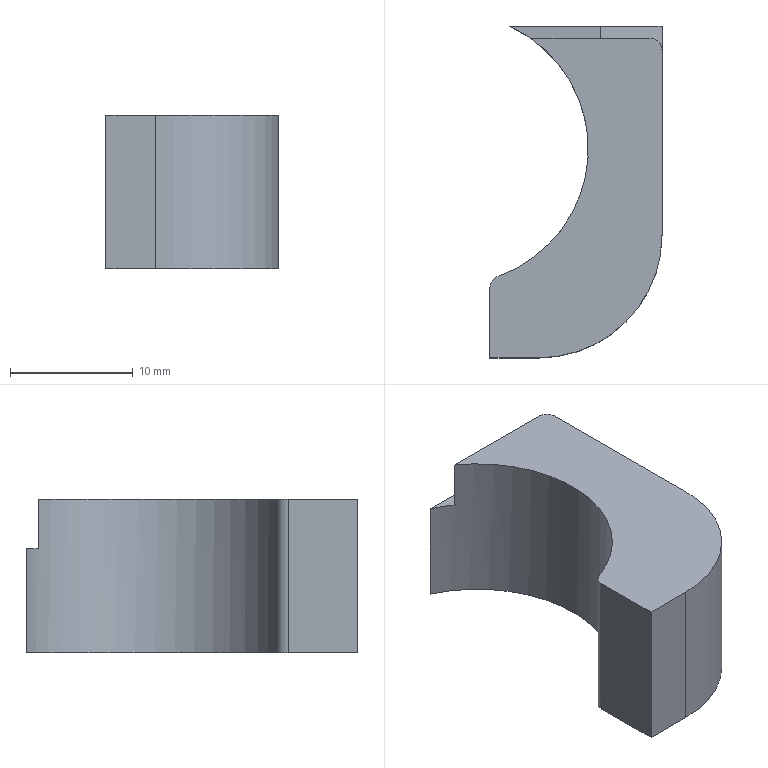Part | SolidWorks | features Fillet 3, Extrusion 1, HoleWzd 1, ICE 1 | 1 solid | 21 faces | box 14 x 27 x 12.5 mm | volume 2830 mm3 | plane 9 | cylinder 8 | cone 4 | commonest cylinder face diameters 1.6 x4 2 x2 20 x1 22 x1
STEP:
#1=CARTESIAN_POINT('',(4.8,2.5,5.2));
#2=VERTEX_POINT('',#1);
#3=CARTESIAN_POINT('',(3.2,2.5,5.2));
#4=VERTEX_POINT('',#3);
#5=CARTESIAN_POINT('',(4.,2.5,5.2));
#6=DIRECTION('',(0.,0.,-1.));
#7=DIRECTION('',(-1.,0.,0.));
#8=AXIS2_PLACEMENT_3D('',#5,#6,#7);
#9=CIRCLE('',#8,0.8);
#10=EDGE_CURVE('',#2,#4,#9,.T.);
#11=ORIENTED_EDGE('',*,*,#10,.F.);
#12=CARTESIAN_POINT('',(4.8,2.5,0.));
#13=VERTEX_POINT('',#12);
#14=CARTESIAN_POINT('',(4.8,2.5,0.));
#15=DIRECTION('',(0.,0.,-1.));
#16=VECTOR('',#15,1000.);
#17=LINE('',#14,#16);
#18=EDGE_CURVE('',#2,#13,#17,.T.);
#19=ORIENTED_EDGE('',*,*,#18,.T.);
#20=CARTESIAN_POINT('',(3.2,2.5,0.));
#21=VERTEX_POINT('',#20);
#22=CARTESIAN_POINT('',(4.,2.5,0.));
#23=DIRECTION('',(0.,0.,-1.));
#24=DIRECTION('',(-1.,0.,0.));
#25=AXIS2_PLACEMENT_3D('',#22,#23,#24);
#26=CIRCLE('',#25,0.8);
#27=EDGE_CURVE('',#13,#21,#26,.T.);
#28=ORIENTED_EDGE('',*,*,#27,.T.);
#29=CARTESIAN_POINT('',(3.2,2.5,0.));
#30=DIRECTION('',(0.,0.,-1.));
#31=VECTOR('',#30,1000.);
#32=LINE('',#29,#31);
#33=EDGE_CURVE('',#4,#21,#32,.T.);
#34=ORIENTED_EDGE('',*,*,#33,.F.);
#35=EDGE_LOOP('',(#11,#19,#28,#34));
#36=FACE_OUTER_BOUND('',#35,.T.);
#37=CARTESIAN_POINT('',(4.,2.5,0.));
#38=DIRECTION('',(0.,0.,-1.));
#39=DIRECTION('',(-1.,0.,0.));
#40=AXIS2_PLACEMENT_3D('',#37,#38,#39);
#41=CYLINDRICAL_SURFACE('',#40,0.8);
#42=ADVANCED_FACE('',(#36),#41,.F.);
#43=CARTESIAN_POINT('',(4.,2.5,5.681));
#44=VERTEX_POINT('',#43);
#45=CARTESIAN_POINT('',(3.2,2.5,5.2));
#46=DIRECTION('',(-0.8572,0.,-0.515));
#47=VECTOR('',#46,1000.);
#48=LINE('',#45,#47);
#49=EDGE_CURVE('',#44,#4,#48,.T.);
#50=ORIENTED_EDGE('',*,*,#49,.F.);
#51=CARTESIAN_POINT('',(4.8,2.5,5.2));
#52=DIRECTION('',(0.8572,0.,-0.515));
#53=VECTOR('',#52,1000.);
#54=LINE('',#51,#53);
#55=EDGE_CURVE('',#44,#2,#54,.T.);
#56=ORIENTED_EDGE('',*,*,#55,.T.);
#57=ORIENTED_EDGE('',*,*,#10,.T.);
#58=EDGE_LOOP('',(#50,#56,#57));
#59=FACE_OUTER_BOUND('',#58,.T.);
#60=CARTESIAN_POINT('',(4.,2.5,5.2));
#61=DIRECTION('',(0.,0.,-1.));
#62=DIRECTION('',(-1.,0.,0.));
#63=AXIS2_PLACEMENT_3D('',#60,#61,#62);
#64=CONICAL_SURFACE('',#63,0.8,1.03);
#65=ADVANCED_FACE('',(#59),#64,.F.);
#66=CARTESIAN_POINT('',(4.8,10.5,5.2));
#67=VERTEX_POINT('',#66);
#68=CARTESIAN_POINT('',(3.2,10.5,5.2));
#69=VERTEX_POINT('',#68);
#70=CARTESIAN_POINT('',(4.,10.5,5.2));
#71=DIRECTION('',(0.,0.,-1.));
#72=DIRECTION('',(-1.,0.,0.));
#73=AXIS2_PLACEMENT_3D('',#70,#71,#72);
#74=CIRCLE('',#73,0.8);
#75=EDGE_CURVE('',#67,#69,#74,.T.);
#76=ORIENTED_EDGE('',*,*,#75,.F.);
#77=CARTESIAN_POINT('',(4.8,10.5,0.));
#78=VERTEX_POINT('',#77);
#79=CARTESIAN_POINT('',(4.8,10.5,0.));
#80=DIRECTION('',(0.,0.,-1.));
#81=VECTOR('',#80,1000.);
#82=LINE('',#79,#81);
#83=EDGE_CURVE('',#67,#78,#82,.T.);
#84=ORIENTED_EDGE('',*,*,#83,.T.);
#85=CARTESIAN_POINT('',(3.2,10.5,0.));
#86=VERTEX_POINT('',#85);
#87=CARTESIAN_POINT('',(4.,10.5,0.));
#88=DIRECTION('',(0.,0.,-1.));
#89=DIRECTION('',(-1.,0.,0.));
#90=AXIS2_PLACEMENT_3D('',#87,#88,#89);
#91=CIRCLE('',#90,0.8);
#92=EDGE_CURVE('',#78,#86,#91,.T.);
#93=ORIENTED_EDGE('',*,*,#92,.T.);
#94=CARTESIAN_POINT('',(3.2,10.5,0.));
#95=DIRECTION('',(0.,0.,-1.));
#96=VECTOR('',#95,1000.);
#97=LINE('',#94,#96);
#98=EDGE_CURVE('',#69,#86,#97,.T.);
#99=ORIENTED_EDGE('',*,*,#98,.F.);
#100=EDGE_LOOP('',(#76,#84,#93,#99));
#101=FACE_OUTER_BOUND('',#100,.T.);
#102=CARTESIAN_POINT('',(4.,10.5,0.));
#103=DIRECTION('',(0.,0.,-1.));
#104=DIRECTION('',(-1.,0.,0.));
#105=AXIS2_PLACEMENT_3D('',#102,#103,#104);
#106=CYLINDRICAL_SURFACE('',#105,0.8);
#107=ADVANCED_FACE('',(#101),#106,.F.);
#108=CARTESIAN_POINT('',(4.,10.5,5.681));
#109=VERTEX_POINT('',#108);
#110=CARTESIAN_POINT('',(3.2,10.5,5.2));
#111=DIRECTION('',(-0.8572,0.,-0.515));
#112=VECTOR('',#111,1000.);
#113=LINE('',#110,#112);
#114=EDGE_CURVE('',#109,#69,#113,.T.);
#115=ORIENTED_EDGE('',*,*,#114,.F.);
#116=CARTESIAN_POINT('',(4.8,10.5,5.2));
#117=DIRECTION('',(0.8572,0.,-0.515));
#118=VECTOR('',#117,1000.);
#119=LINE('',#116,#118);
#120=EDGE_CURVE('',#109,#67,#119,.T.);
#121=ORIENTED_EDGE('',*,*,#120,.T.);
#122=ORIENTED_EDGE('',*,*,#75,.T.);
#123=EDGE_LOOP('',(#115,#121,#122));
#124=FACE_OUTER_BOUND('',#123,.T.);
#125=CARTESIAN_POINT('',(4.,10.5,5.2));
#126=DIRECTION('',(0.,0.,-1.));
#127=DIRECTION('',(-1.,0.,0.));
#128=AXIS2_PLACEMENT_3D('',#125,#126,#127);
#129=CONICAL_SURFACE('',#128,0.8,1.03);
#130=ADVANCED_FACE('',(#124),#129,.F.);
#131=CARTESIAN_POINT('',(-7.,-13.5,0.));
#132=VERTEX_POINT('',#131);
#133=CARTESIAN_POINT('',(-3.,-13.5,0.));
#134=VERTEX_POINT('',#133);
#135=CARTESIAN_POINT('',(7.,-13.5,0.));
#136=DIRECTION('',(1.,0.,0.));
#137=VECTOR('',#136,1000.);
#138=LINE('',#135,#137);
#139=EDGE_CURVE('',#132,#134,#138,.T.);
#140=ORIENTED_EDGE('',*,*,#139,.T.);
#141=CARTESIAN_POINT('',(-3.,-13.5,12.5));
#142=VERTEX_POINT('',#141);
#143=CARTESIAN_POINT('',(-3.,-13.5,12.5));
#144=DIRECTION('',(0.,0.,1.));
#145=VECTOR('',#144,1000.);
#146=LINE('',#143,#145);
#147=EDGE_CURVE('',#134,#142,#146,.T.);
#148=ORIENTED_EDGE('',*,*,#147,.T.);
#149=CARTESIAN_POINT('',(-7.,-13.5,12.5));
#150=VERTEX_POINT('',#149);
#151=CARTESIAN_POINT('',(7.,-13.5,12.5));
#152=DIRECTION('',(1.,0.,0.));
#153=VECTOR('',#152,1000.);
#154=LINE('',#151,#153);
#155=EDGE_CURVE('',#150,#142,#154,.T.);
#156=ORIENTED_EDGE('',*,*,#155,.F.);
#157=CARTESIAN_POINT('',(-7.,-13.5,12.5));
#158=DIRECTION('',(0.,0.,-1.));
#159=VECTOR('',#158,1000.);
#160=LINE('',#157,#159);
#161=EDGE_CURVE('',#150,#132,#160,.T.);
#162=ORIENTED_EDGE('',*,*,#161,.T.);
#163=EDGE_LOOP('',(#140,#148,#156,#162));
#164=FACE_OUTER_BOUND('',#163,.T.);
#165=CARTESIAN_POINT('',(7.,-13.5,12.5));
#166=DIRECTION('',(0.,1.,0.));
#167=DIRECTION('',(-1.,0.,0.));
#168=AXIS2_PLACEMENT_3D('',#165,#166,#167);
#169=PLANE('',#168);
#170=ADVANCED_FACE('',(#164),#169,.F.);
#171=CARTESIAN_POINT('',(7.,11.5,7.5));
#172=VERTEX_POINT('',#171);
#173=CARTESIAN_POINT('',(7.,13.5,7.5));
#174=VERTEX_POINT('',#173);
#175=CARTESIAN_POINT('',(7.,12.5,7.5));
#176=DIRECTION('',(0.,1.,0.));
#177=VECTOR('',#176,1000.);
#178=LINE('',#175,#177);
#179=EDGE_CURVE('',#172,#174,#178,.T.);
#180=ORIENTED_EDGE('',*,*,#179,.F.);
#181=CARTESIAN_POINT('',(7.,11.5,12.5));
#182=VERTEX_POINT('',#181);
#183=CARTESIAN_POINT('',(7.,11.5,12.5));
#184=DIRECTION('',(0.,0.,1.));
#185=VECTOR('',#184,1000.);
#186=LINE('',#183,#185);
#187=EDGE_CURVE('',#172,#182,#186,.T.);
#188=ORIENTED_EDGE('',*,*,#187,.T.);
#189=CARTESIAN_POINT('',(7.,-3.5,12.5));
#190=VERTEX_POINT('',#189);
#191=CARTESIAN_POINT('',(7.,13.5,12.5));
#192=DIRECTION('',(0.,1.,0.));
#193=VECTOR('',#192,1000.);
#194=LINE('',#191,#193);
#195=EDGE_CURVE('',#190,#182,#194,.T.);
#196=ORIENTED_EDGE('',*,*,#195,.F.);
#197=CARTESIAN_POINT('',(7.,-3.5,0.));
#198=VERTEX_POINT('',#197);
#199=CARTESIAN_POINT('',(7.,-3.5,12.5));
#200=DIRECTION('',(0.,0.,-1.));
#201=VECTOR('',#200,1000.);
#202=LINE('',#199,#201);
#203=EDGE_CURVE('',#190,#198,#202,.T.);
#204=ORIENTED_EDGE('',*,*,#203,.T.);
#205=CARTESIAN_POINT('',(7.,13.5,0.));
#206=VERTEX_POINT('',#205);
#207=CARTESIAN_POINT('',(7.,13.5,0.));
#208=DIRECTION('',(0.,1.,0.));
#209=VECTOR('',#208,1000.);
#210=LINE('',#207,#209);
#211=EDGE_CURVE('',#198,#206,#210,.T.);
#212=ORIENTED_EDGE('',*,*,#211,.T.);
#213=CARTESIAN_POINT('',(7.,13.5,12.5));
#214=DIRECTION('',(0.,0.,-1.));
#215=VECTOR('',#214,1000.);
#216=LINE('',#213,#215);
#217=EDGE_CURVE('',#174,#206,#216,.T.);
#218=ORIENTED_EDGE('',*,*,#217,.F.);
#219=EDGE_LOOP('',(#180,#188,#196,#204,#212,#218));
#220=FACE_OUTER_BOUND('',#219,.T.);
#221=CARTESIAN_POINT('',(7.,13.5,12.5));
#222=DIRECTION('',(-1.,0.,0.));
#223=DIRECTION('',(0.,-1.,0.));
#224=AXIS2_PLACEMENT_3D('',#221,#222,#223);
#225=PLANE('',#224);
#226=ADVANCED_FACE('',(#220),#225,.F.);
#227=CARTESIAN_POINT('',(-5.417,13.5,8.5));
#228=VERTEX_POINT('',#227);
#229=CARTESIAN_POINT('',(-5.417,13.5,0.));
#230=VERTEX_POINT('',#229);
#231=CARTESIAN_POINT('',(-5.417,13.5,12.5));
#232=DIRECTION('',(0.,0.,-1.));
#233=VECTOR('',#232,1000.);
#234=LINE('',#231,#233);
#235=EDGE_CURVE('',#228,#230,#234,.T.);
#236=ORIENTED_EDGE('',*,*,#235,.F.);
#237=CARTESIAN_POINT('',(2.,13.5,8.5));
#238=VERTEX_POINT('',#237);
#239=CARTESIAN_POINT('',(-5.417,13.5,8.5));
#240=DIRECTION('',(-1.,0.,0.));
#241=VECTOR('',#240,1000.);
#242=LINE('',#239,#241);
#243=EDGE_CURVE('',#238,#228,#242,.T.);
#244=ORIENTED_EDGE('',*,*,#243,.F.);
#245=CARTESIAN_POINT('',(2.,13.5,8.5));
#246=DIRECTION('',(-0.9806,0.,0.1961));
#247=VECTOR('',#246,1000.);
#248=LINE('',#245,#247);
#249=EDGE_CURVE('',#174,#238,#248,.T.);
#250=ORIENTED_EDGE('',*,*,#249,.F.);
#251=ORIENTED_EDGE('',*,*,#217,.T.);
#252=CARTESIAN_POINT('',(7.,13.5,0.));
#253=DIRECTION('',(-1.,0.,0.));
#254=VECTOR('',#253,1000.);
#255=LINE('',#252,#254);
#256=EDGE_CURVE('',#206,#230,#255,.T.);
#257=ORIENTED_EDGE('',*,*,#256,.T.);
#258=EDGE_LOOP('',(#236,#244,#250,#251,#257));
#259=FACE_OUTER_BOUND('',#258,.T.);
#260=CARTESIAN_POINT('',(7.,13.5,12.5));
#261=DIRECTION('',(0.,-1.,0.));
#262=DIRECTION('',(1.,0.,0.));
#263=AXIS2_PLACEMENT_3D('',#260,#261,#262);
#264=PLANE('',#263);
#265=ADVANCED_FACE('',(#259),#264,.F.);
#266=CARTESIAN_POINT('',(-6.333,-6.871,0.));
#267=VERTEX_POINT('',#266);
#268=CARTESIAN_POINT('',(-10.,3.5,0.));
#269=DIRECTION('',(0.,0.,-1.));
#270=DIRECTION('',(1.,0.,0.));
#271=AXIS2_PLACEMENT_3D('',#268,#269,#270);
#272=CIRCLE('',#271,11.);
#273=EDGE_CURVE('',#230,#267,#272,.T.);
#274=ORIENTED_EDGE('',*,*,#273,.T.);
#275=CARTESIAN_POINT('',(-6.333,-6.871,12.5));
#276=VERTEX_POINT('',#275);
#277=CARTESIAN_POINT('',(-6.333,-6.871,12.5));
#278=DIRECTION('',(0.,0.,1.));
#279=VECTOR('',#278,1000.);
#280=LINE('',#277,#279);
#281=EDGE_CURVE('',#267,#276,#280,.T.);
#282=ORIENTED_EDGE('',*,*,#281,.T.);
#283=CARTESIAN_POINT('',(-3.675,12.5,12.5));
#284=VERTEX_POINT('',#283);
#285=CARTESIAN_POINT('',(-10.,3.5,12.5));
#286=DIRECTION('',(0.,0.,-1.));
#287=DIRECTION('',(1.,0.,0.));
#288=AXIS2_PLACEMENT_3D('',#285,#286,#287);
#289=CIRCLE('',#288,11.);
#290=EDGE_CURVE('',#284,#276,#289,.T.);
#291=ORIENTED_EDGE('',*,*,#290,.F.);
#292=CARTESIAN_POINT('',(-3.675,12.5,8.5));
#293=VERTEX_POINT('',#292);
#294=CARTESIAN_POINT('',(-3.675,12.5,12.5));
#295=DIRECTION('',(0.,0.,-1.));
#296=VECTOR('',#295,1000.);
#297=LINE('',#294,#296);
#298=EDGE_CURVE('',#284,#293,#297,.T.);
#299=ORIENTED_EDGE('',*,*,#298,.T.);
#300=CARTESIAN_POINT('',(-10.,3.5,8.5));
#301=DIRECTION('',(0.,0.,1.));
#302=DIRECTION('',(-1.,0.,0.));
#303=AXIS2_PLACEMENT_3D('',#300,#301,#302);
#304=CIRCLE('',#303,11.);
#305=EDGE_CURVE('',#293,#228,#304,.T.);
#306=ORIENTED_EDGE('',*,*,#305,.T.);
#307=ORIENTED_EDGE('',*,*,#235,.T.);
#308=EDGE_LOOP('',(#274,#282,#291,#299,#306,#307));
#309=FACE_OUTER_BOUND('',#308,.T.);
#310=CARTESIAN_POINT('',(-10.,3.5,12.5));
#311=DIRECTION('',(0.,0.,-1.));
#312=DIRECTION('',(-1.,0.,0.));
#313=AXIS2_PLACEMENT_3D('',#310,#311,#312);
#314=CYLINDRICAL_SURFACE('',#313,11.);
#315=ADVANCED_FACE('',(#309),#314,.F.);
#316=CARTESIAN_POINT('',(-7.,-7.814,12.5));
#317=VERTEX_POINT('',#316);
#318=CARTESIAN_POINT('',(-7.,-7.083,12.5));
#319=DIRECTION('',(0.,-1.,0.));
#320=VECTOR('',#319,1000.);
#321=LINE('',#318,#320);
#322=EDGE_CURVE('',#317,#150,#321,.T.);
#323=ORIENTED_EDGE('',*,*,#322,.F.);
#324=CARTESIAN_POINT('',(-7.,-7.814,0.));
#325=VERTEX_POINT('',#324);
#326=CARTESIAN_POINT('',(-7.,-7.814,12.5));
#327=DIRECTION('',(0.,0.,-1.));
#328=VECTOR('',#327,1000.);
#329=LINE('',#326,#328);
#330=EDGE_CURVE('',#317,#325,#329,.T.);
#331=ORIENTED_EDGE('',*,*,#330,.T.);
#332=CARTESIAN_POINT('',(-7.,-7.083,0.));
#333=DIRECTION('',(0.,-1.,0.));
#334=VECTOR('',#333,1000.);
#335=LINE('',#332,#334);
#336=EDGE_CURVE('',#325,#132,#335,.T.);
#337=ORIENTED_EDGE('',*,*,#336,.T.);
#338=ORIENTED_EDGE('',*,*,#161,.F.);
#339=EDGE_LOOP('',(#323,#331,#337,#338));
#340=FACE_OUTER_BOUND('',#339,.T.);
#341=CARTESIAN_POINT('',(-7.,-7.083,12.5));
#342=DIRECTION('',(1.,0.,0.));
#343=DIRECTION('',(0.,1.,0.));
#344=AXIS2_PLACEMENT_3D('',#341,#342,#343);
#345=PLANE('',#344);
#346=ADVANCED_FACE('',(#340),#345,.F.);
#347=ORIENTED_EDGE('',*,*,#290,.T.);
#348=CARTESIAN_POINT('',(-6.,-7.814,12.5));
#349=DIRECTION('',(0.,0.,1.));
#350=DIRECTION('',(1.,0.,0.));
#351=AXIS2_PLACEMENT_3D('',#348,#349,#350);
#352=CIRCLE('',#351,1.);
#353=EDGE_CURVE('',#276,#317,#352,.T.);
#354=ORIENTED_EDGE('',*,*,#353,.T.);
#355=ORIENTED_EDGE('',*,*,#322,.T.);
#356=ORIENTED_EDGE('',*,*,#155,.T.);
#357=CARTESIAN_POINT('',(-3.,-3.5,12.5));
#358=DIRECTION('',(0.,0.,1.));
#359=DIRECTION('',(1.,0.,0.));
#360=AXIS2_PLACEMENT_3D('',#357,#358,#359);
#361=CIRCLE('',#360,10.);
#362=EDGE_CURVE('',#142,#190,#361,.T.);
#363=ORIENTED_EDGE('',*,*,#362,.T.);
#364=ORIENTED_EDGE('',*,*,#195,.T.);
#365=CARTESIAN_POINT('',(6.,12.5,12.5));
#366=VERTEX_POINT('',#365);
#367=CARTESIAN_POINT('',(6.,11.5,12.5));
#368=DIRECTION('',(0.,0.,1.));
#369=DIRECTION('',(1.,0.,0.));
#370=AXIS2_PLACEMENT_3D('',#367,#368,#369);
#371=CIRCLE('',#370,1.);
#372=EDGE_CURVE('',#182,#366,#371,.T.);
#373=ORIENTED_EDGE('',*,*,#372,.T.);
#374=CARTESIAN_POINT('',(-10.,12.5,12.5));
#375=DIRECTION('',(1.,0.,0.));
#376=VECTOR('',#375,1000.);
#377=LINE('',#374,#376);
#378=EDGE_CURVE('',#284,#366,#377,.T.);
#379=ORIENTED_EDGE('',*,*,#378,.F.);
#380=EDGE_LOOP('',(#347,#354,#355,#356,#363,#364,#373,#379));
#381=FACE_OUTER_BOUND('',#380,.T.);
#382=CARTESIAN_POINT('',(-10.,3.5,12.5));
#383=DIRECTION('',(0.,0.,1.));
#384=DIRECTION('',(1.,0.,0.));
#385=AXIS2_PLACEMENT_3D('',#382,#383,#384);
#386=PLANE('',#385);
#387=ADVANCED_FACE('',(#381),#386,.T.);
#388=CARTESIAN_POINT('',(4.,2.5,0.));
#389=DIRECTION('',(0.,0.,-1.));
#390=DIRECTION('',(-1.,0.,0.));
#391=AXIS2_PLACEMENT_3D('',#388,#389,#390);
#392=CIRCLE('',#391,0.8);
#393=EDGE_CURVE('',#21,#13,#392,.T.);
#394=ORIENTED_EDGE('',*,*,#393,.F.);
#395=ORIENTED_EDGE('',*,*,#27,.F.);
#396=EDGE_LOOP('',(#394,#395));
#397=FACE_BOUND('',#396,.T.);
#398=CARTESIAN_POINT('',(4.,10.5,0.));
#399=DIRECTION('',(0.,0.,-1.));
#400=DIRECTION('',(-1.,0.,0.));
#401=AXIS2_PLACEMENT_3D('',#398,#399,#400);
#402=CIRCLE('',#401,0.8);
#403=EDGE_CURVE('',#86,#78,#402,.T.);
#404=ORIENTED_EDGE('',*,*,#403,.F.);
#405=ORIENTED_EDGE('',*,*,#92,.F.);
#406=EDGE_LOOP('',(#404,#405));
#407=FACE_BOUND('',#406,.T.);
#408=ORIENTED_EDGE('',*,*,#336,.F.);
#409=CARTESIAN_POINT('',(-6.,-7.814,0.));
#410=DIRECTION('',(0.,0.,-1.));
#411=DIRECTION('',(1.,0.,0.));
#412=AXIS2_PLACEMENT_3D('',#409,#410,#411);
#413=CIRCLE('',#412,1.);
#414=EDGE_CURVE('',#325,#267,#413,.T.);
#415=ORIENTED_EDGE('',*,*,#414,.T.);
#416=ORIENTED_EDGE('',*,*,#273,.F.);
#417=ORIENTED_EDGE('',*,*,#256,.F.);
#418=ORIENTED_EDGE('',*,*,#211,.F.);
#419=CARTESIAN_POINT('',(-3.,-3.5,0.));
#420=DIRECTION('',(0.,0.,-1.));
#421=DIRECTION('',(1.,0.,0.));
#422=AXIS2_PLACEMENT_3D('',#419,#420,#421);
#423=CIRCLE('',#422,10.);
#424=EDGE_CURVE('',#198,#134,#423,.T.);
#425=ORIENTED_EDGE('',*,*,#424,.T.);
#426=ORIENTED_EDGE('',*,*,#139,.F.);
#427=EDGE_LOOP('',(#408,#415,#416,#417,#418,#425,#426));
#428=FACE_OUTER_BOUND('',#427,.T.);
#429=CARTESIAN_POINT('',(-10.,3.5,0.));
#430=DIRECTION('',(0.,0.,1.));
#431=DIRECTION('',(1.,0.,0.));
#432=AXIS2_PLACEMENT_3D('',#429,#430,#431);
#433=PLANE('',#432);
#434=ADVANCED_FACE('',(#397,#407,#428),#433,.F.);
#435=CARTESIAN_POINT('',(2.,12.5,8.5));
#436=VERTEX_POINT('',#435);
#437=CARTESIAN_POINT('',(-5.417,12.5,8.5));
#438=DIRECTION('',(-1.,0.,0.));
#439=VECTOR('',#438,1000.);
#440=LINE('',#437,#439);
#441=EDGE_CURVE('',#436,#293,#440,.T.);
#442=ORIENTED_EDGE('',*,*,#441,.F.);
#443=CARTESIAN_POINT('',(2.,12.5,8.5));
#444=DIRECTION('',(0.,1.,0.));
#445=VECTOR('',#444,1000.);
#446=LINE('',#443,#445);
#447=EDGE_CURVE('',#436,#238,#446,.T.);
#448=ORIENTED_EDGE('',*,*,#447,.T.);
#449=ORIENTED_EDGE('',*,*,#243,.T.);
#450=ORIENTED_EDGE('',*,*,#305,.F.);
#451=EDGE_LOOP('',(#442,#448,#449,#450));
#452=FACE_OUTER_BOUND('',#451,.T.);
#453=CARTESIAN_POINT('',(-5.417,12.5,8.5));
#454=DIRECTION('',(0.,0.,-1.));
#455=DIRECTION('',(-1.,0.,0.));
#456=AXIS2_PLACEMENT_3D('',#453,#454,#455);
#457=PLANE('',#456);
#458=ADVANCED_FACE('',(#452),#457,.F.);
#459=ORIENTED_EDGE('',*,*,#378,.T.);
#460=CARTESIAN_POINT('',(6.,12.5,7.7));
#461=VERTEX_POINT('',#460);
#462=CARTESIAN_POINT('',(6.,12.5,0.));
#463=DIRECTION('',(0.,0.,-1.));
#464=VECTOR('',#463,1000.);
#465=LINE('',#462,#464);
#466=EDGE_CURVE('',#366,#461,#465,.T.);
#467=ORIENTED_EDGE('',*,*,#466,.T.);
#468=CARTESIAN_POINT('',(2.,12.5,8.5));
#469=DIRECTION('',(-0.9806,0.,0.1961));
#470=VECTOR('',#469,1000.);
#471=LINE('',#468,#470);
#472=EDGE_CURVE('',#461,#436,#471,.T.);
#473=ORIENTED_EDGE('',*,*,#472,.T.);
#474=ORIENTED_EDGE('',*,*,#441,.T.);
#475=ORIENTED_EDGE('',*,*,#298,.F.);
#476=EDGE_LOOP('',(#459,#467,#473,#474,#475));
#477=FACE_OUTER_BOUND('',#476,.T.);
#478=CARTESIAN_POINT('',(0.,12.5,0.));
#479=DIRECTION('',(0.,-1.,0.));
#480=DIRECTION('',(1.,0.,0.));
#481=AXIS2_PLACEMENT_3D('',#478,#479,#480);
#482=PLANE('',#481);
#483=ADVANCED_FACE('',(#477),#482,.F.);
#484=ORIENTED_EDGE('',*,*,#249,.T.);
#485=ORIENTED_EDGE('',*,*,#447,.F.);
#486=ORIENTED_EDGE('',*,*,#472,.F.);
#487=CARTESIAN_POINT('',(6.,12.5,7.7));
#488=CARTESIAN_POINT('',(6.586,12.5,7.583));
#489=CARTESIAN_POINT('',(7.,12.086,7.5));
#490=CARTESIAN_POINT('',(7.,11.5,7.5));
#491=(BOUNDED_CURVE()B_SPLINE_CURVE(3,(#487,#488,#489,#490),.UNSPECIFIED.,.F.,.F.)B_SPLINE_CURVE_WITH_KNOTS((4,4),(4.712,6.283),.UNSPECIFIED.)CURVE()GEOMETRIC_REPRESENTATION_ITEM()RATIONAL_B_SPLINE_CURVE((1.,0.8047,0.8047,1.))REPRESENTATION_ITEM(''));
#492=EDGE_CURVE('',#461,#172,#491,.T.);
#493=ORIENTED_EDGE('',*,*,#492,.T.);
#494=ORIENTED_EDGE('',*,*,#179,.T.);
#495=EDGE_LOOP('',(#484,#485,#486,#493,#494));
#496=FACE_OUTER_BOUND('',#495,.T.);
#497=CARTESIAN_POINT('',(2.,12.5,8.5));
#498=DIRECTION('',(-0.1961,0.,-0.9806));
#499=DIRECTION('',(-0.9806,0.,0.1961));
#500=AXIS2_PLACEMENT_3D('',#497,#498,#499);
#501=PLANE('',#500);
#502=ADVANCED_FACE('',(#496),#501,.F.);
#503=ORIENTED_EDGE('',*,*,#362,.F.);
#504=ORIENTED_EDGE('',*,*,#147,.F.);
#505=ORIENTED_EDGE('',*,*,#424,.F.);
#506=ORIENTED_EDGE('',*,*,#203,.F.);
#507=EDGE_LOOP('',(#503,#504,#505,#506));
#508=FACE_OUTER_BOUND('',#507,.T.);
#509=CARTESIAN_POINT('',(-3.,-3.5,12.5));
#510=DIRECTION('',(0.,0.,-1.));
#511=DIRECTION('',(-1.,0.,0.));
#512=AXIS2_PLACEMENT_3D('',#509,#510,#511);
#513=CYLINDRICAL_SURFACE('',#512,10.);
#514=ADVANCED_FACE('',(#508),#513,.T.);
#515=ORIENTED_EDGE('',*,*,#372,.F.);
#516=ORIENTED_EDGE('',*,*,#187,.F.);
#517=ORIENTED_EDGE('',*,*,#492,.F.);
#518=ORIENTED_EDGE('',*,*,#466,.F.);
#519=EDGE_LOOP('',(#515,#516,#517,#518));
#520=FACE_OUTER_BOUND('',#519,.T.);
#521=CARTESIAN_POINT('',(6.,11.5,0.));
#522=DIRECTION('',(0.,0.,-1.));
#523=DIRECTION('',(-1.,0.,0.));
#524=AXIS2_PLACEMENT_3D('',#521,#522,#523);
#525=CYLINDRICAL_SURFACE('',#524,1.);
#526=ADVANCED_FACE('',(#520),#525,.T.);
#527=ORIENTED_EDGE('',*,*,#120,.F.);
#528=ORIENTED_EDGE('',*,*,#114,.T.);
#529=CARTESIAN_POINT('',(4.,10.5,5.2));
#530=DIRECTION('',(0.,0.,-1.));
#531=DIRECTION('',(-1.,0.,0.));
#532=AXIS2_PLACEMENT_3D('',#529,#530,#531);
#533=CIRCLE('',#532,0.8);
#534=EDGE_CURVE('',#69,#67,#533,.T.);
#535=ORIENTED_EDGE('',*,*,#534,.T.);
#536=EDGE_LOOP('',(#527,#528,#535));
#537=FACE_OUTER_BOUND('',#536,.T.);
#538=CARTESIAN_POINT('',(4.,10.5,5.2));
#539=DIRECTION('',(0.,0.,-1.));
#540=DIRECTION('',(-1.,0.,0.));
#541=AXIS2_PLACEMENT_3D('',#538,#539,#540);
#542=CONICAL_SURFACE('',#541,0.8,1.03);
#543=ADVANCED_FACE('',(#537),#542,.F.);
#544=ORIENTED_EDGE('',*,*,#83,.F.);
#545=ORIENTED_EDGE('',*,*,#534,.F.);
#546=ORIENTED_EDGE('',*,*,#98,.T.);
#547=ORIENTED_EDGE('',*,*,#403,.T.);
#548=EDGE_LOOP('',(#544,#545,#546,#547));
#549=FACE_OUTER_BOUND('',#548,.T.);
#550=CARTESIAN_POINT('',(4.,10.5,0.));
#551=DIRECTION('',(0.,0.,-1.));
#552=DIRECTION('',(-1.,0.,0.));
#553=AXIS2_PLACEMENT_3D('',#550,#551,#552);
#554=CYLINDRICAL_SURFACE('',#553,0.8);
#555=ADVANCED_FACE('',(#549),#554,.F.);
#556=ORIENTED_EDGE('',*,*,#55,.F.);
#557=ORIENTED_EDGE('',*,*,#49,.T.);
#558=CARTESIAN_POINT('',(4.,2.5,5.2));
#559=DIRECTION('',(0.,0.,-1.));
#560=DIRECTION('',(-1.,0.,0.));
#561=AXIS2_PLACEMENT_3D('',#558,#559,#560);
#562=CIRCLE('',#561,0.8);
#563=EDGE_CURVE('',#4,#2,#562,.T.);
#564=ORIENTED_EDGE('',*,*,#563,.T.);
#565=EDGE_LOOP('',(#556,#557,#564));
#566=FACE_OUTER_BOUND('',#565,.T.);
#567=CARTESIAN_POINT('',(4.,2.5,5.2));
#568=DIRECTION('',(0.,0.,-1.));
#569=DIRECTION('',(-1.,0.,0.));
#570=AXIS2_PLACEMENT_3D('',#567,#568,#569);
#571=CONICAL_SURFACE('',#570,0.8,1.03);
#572=ADVANCED_FACE('',(#566),#571,.F.);
#573=ORIENTED_EDGE('',*,*,#18,.F.);
#574=ORIENTED_EDGE('',*,*,#563,.F.);
#575=ORIENTED_EDGE('',*,*,#33,.T.);
#576=ORIENTED_EDGE('',*,*,#393,.T.);
#577=EDGE_LOOP('',(#573,#574,#575,#576));
#578=FACE_OUTER_BOUND('',#577,.T.);
#579=CARTESIAN_POINT('',(4.,2.5,0.));
#580=DIRECTION('',(0.,0.,-1.));
#581=DIRECTION('',(-1.,0.,0.));
#582=AXIS2_PLACEMENT_3D('',#579,#580,#581);
#583=CYLINDRICAL_SURFACE('',#582,0.8);
#584=ADVANCED_FACE('',(#578),#583,.F.);
#585=ORIENTED_EDGE('',*,*,#353,.F.);
#586=ORIENTED_EDGE('',*,*,#281,.F.);
#587=ORIENTED_EDGE('',*,*,#414,.F.);
#588=ORIENTED_EDGE('',*,*,#330,.F.);
#589=EDGE_LOOP('',(#585,#586,#587,#588));
#590=FACE_OUTER_BOUND('',#589,.T.);
#591=CARTESIAN_POINT('',(-6.,-7.814,12.5));
#592=DIRECTION('',(0.,0.,-1.));
#593=DIRECTION('',(-1.,0.,0.));
#594=AXIS2_PLACEMENT_3D('',#591,#592,#593);
#595=CYLINDRICAL_SURFACE('',#594,1.);
#596=ADVANCED_FACE('',(#590),#595,.T.);
#597=CLOSED_SHELL('',(#42,#65,#107,#130,#170,#226,#265,#315,#346,#387,#434,#458,#483,#502,#514,#526,#543,#555,#572,#584,#596));
#598=MANIFOLD_SOLID_BREP('',#597);
#599=CARTESIAN_POINT('',(0.,0.,0.));
#600=DIRECTION('',(0.,0.,1.));
#601=DIRECTION('',(1.,0.,0.));
#602=AXIS2_PLACEMENT_3D('',#599,#600,#601);
#603=(LENGTH_UNIT()NAMED_UNIT(*)SI_UNIT(.MILLI.,.METRE.));
#604=UNCERTAINTY_MEASURE_WITH_UNIT(LENGTH_MEASURE(0.00001),#603,'','');
#605=(NAMED_UNIT(*)PLANE_ANGLE_UNIT()SI_UNIT($,.RADIAN.));
#606=(NAMED_UNIT(*)SI_UNIT($,.STERADIAN.)SOLID_ANGLE_UNIT());
#607=(GEOMETRIC_REPRESENTATION_CONTEXT(3)GLOBAL_UNCERTAINTY_ASSIGNED_CONTEXT((#604))GLOBAL_UNIT_ASSIGNED_CONTEXT((#603,#605,#606))REPRESENTATION_CONTEXT('',''));
#608=ADVANCED_BREP_SHAPE_REPRESENTATION('',(#598,#602),#607);